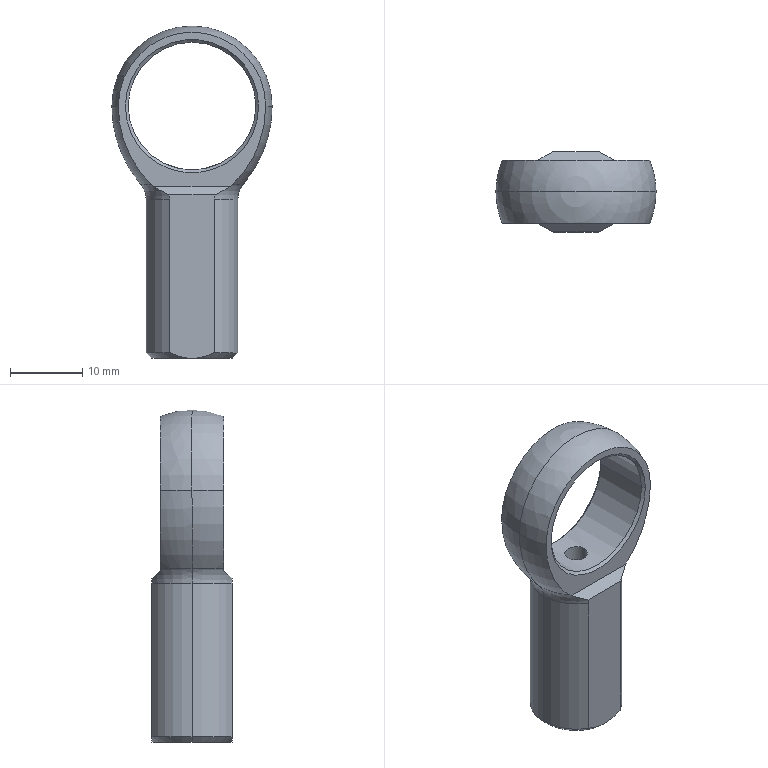Part | NX | features LUMP1 2 | 1 solid | 42 faces | box 22.225 x 11.1 x 46.038 mm | volume 3030 mm3 | cylinder 12 | cone 12 | plane 8 | torus 8 | sphere 2 | commonest cylinder face diameters 12.7 x4 3.175 x2 6.678 x2 7.938 x2 17.704 x2
STEP:
#1=CARTESIAN_POINT('',(3.339,0.,19.05));
#2=VERTEX_POINT('',#1);
#3=CARTESIAN_POINT('',(-3.339,0.,19.05));
#4=VERTEX_POINT('',#3);
#5=CARTESIAN_POINT('',(0.,0.,19.05));
#6=DIRECTION('',(0.,0.,-1.));
#7=DIRECTION('',(1.,0.,0.));
#8=AXIS2_PLACEMENT_3D('',#5,#6,#7);
#9=CIRCLE('',#8,3.339);
#10=EDGE_CURVE('',#2,#4,#9,.T.);
#11=ORIENTED_EDGE('',*,*,#10,.F.);
#12=CARTESIAN_POINT('',(0.,0.,19.05));
#13=DIRECTION('',(0.,0.,-1.));
#14=DIRECTION('',(1.,0.,0.));
#15=AXIS2_PLACEMENT_3D('',#12,#13,#14);
#16=CIRCLE('',#15,3.339);
#17=EDGE_CURVE('',#4,#2,#16,.T.);
#18=ORIENTED_EDGE('',*,*,#17,.F.);
#19=EDGE_LOOP('',(#11,#18));
#20=FACE_BOUND('',#19,.T.);
#21=CARTESIAN_POINT('',(3.969,0.,19.05));
#22=VERTEX_POINT('',#21);
#23=CARTESIAN_POINT('',(-3.969,0.,19.05));
#24=VERTEX_POINT('',#23);
#25=CARTESIAN_POINT('',(0.,0.,19.05));
#26=DIRECTION('',(0.,0.,1.));
#27=DIRECTION('',(1.,0.,0.));
#28=AXIS2_PLACEMENT_3D('',#25,#26,#27);
#29=CIRCLE('',#28,3.969);
#30=EDGE_CURVE('',#22,#24,#29,.T.);
#31=ORIENTED_EDGE('',*,*,#30,.F.);
#32=CARTESIAN_POINT('',(0.,0.,19.05));
#33=DIRECTION('',(0.,0.,1.));
#34=DIRECTION('',(1.,0.,0.));
#35=AXIS2_PLACEMENT_3D('',#32,#33,#34);
#36=CIRCLE('',#35,3.969);
#37=EDGE_CURVE('',#24,#22,#36,.T.);
#38=ORIENTED_EDGE('',*,*,#37,.F.);
#39=EDGE_LOOP('',(#31,#38));
#40=FACE_BOUND('',#39,.T.);
#41=CARTESIAN_POINT('',(0.,0.,19.05));
#42=DIRECTION('',(0.,0.,1.));
#43=DIRECTION('',(-1.,0.,0.));
#44=AXIS2_PLACEMENT_3D('',#41,#42,#43);
#45=PLANE('',#44);
#46=ADVANCED_FACE('',(#20,#40),#45,.F.);
#47=CARTESIAN_POINT('',(3.339,0.,22.225));
#48=VERTEX_POINT('',#47);
#49=CARTESIAN_POINT('',(3.339,0.,20.637));
#50=DIRECTION('',(0.,0.,1.));
#51=VECTOR('',#50,1000.);
#52=LINE('',#49,#51);
#53=EDGE_CURVE('',#2,#48,#52,.T.);
#54=ORIENTED_EDGE('',*,*,#53,.F.);
#55=ORIENTED_EDGE('',*,*,#10,.T.);
#56=CARTESIAN_POINT('',(-3.339,0.,22.225));
#57=VERTEX_POINT('',#56);
#58=CARTESIAN_POINT('',(-3.339,0.,20.637));
#59=DIRECTION('',(0.,0.,-1.));
#60=VECTOR('',#59,1000.);
#61=LINE('',#58,#60);
#62=EDGE_CURVE('',#57,#4,#61,.T.);
#63=ORIENTED_EDGE('',*,*,#62,.F.);
#64=CARTESIAN_POINT('',(0.,0.,22.225));
#65=DIRECTION('',(0.,0.,-1.));
#66=DIRECTION('',(1.,0.,0.));
#67=AXIS2_PLACEMENT_3D('',#64,#65,#66);
#68=CIRCLE('',#67,3.339);
#69=EDGE_CURVE('',#48,#57,#68,.T.);
#70=ORIENTED_EDGE('',*,*,#69,.F.);
#71=EDGE_LOOP('',(#54,#55,#63,#70));
#72=FACE_BOUND('',#71,.T.);
#73=CARTESIAN_POINT('',(0.,0.,20.637));
#74=DIRECTION('',(0.,0.,-1.));
#75=DIRECTION('',(-1.,0.,0.));
#76=AXIS2_PLACEMENT_3D('',#73,#74,#75);
#77=CYLINDRICAL_SURFACE('',#76,3.339);
#78=ADVANCED_FACE('',(#72),#77,.F.);
#79=ORIENTED_EDGE('',*,*,#53,.T.);
#80=CARTESIAN_POINT('',(0.,0.,22.225));
#81=DIRECTION('',(0.,0.,-1.));
#82=DIRECTION('',(1.,0.,0.));
#83=AXIS2_PLACEMENT_3D('',#80,#81,#82);
#84=CIRCLE('',#83,3.339);
#85=EDGE_CURVE('',#57,#48,#84,.T.);
#86=ORIENTED_EDGE('',*,*,#85,.F.);
#87=ORIENTED_EDGE('',*,*,#62,.T.);
#88=ORIENTED_EDGE('',*,*,#17,.T.);
#89=EDGE_LOOP('',(#79,#86,#87,#88));
#90=FACE_BOUND('',#89,.T.);
#91=CARTESIAN_POINT('',(0.,0.,20.637));
#92=DIRECTION('',(0.,0.,-1.));
#93=DIRECTION('',(-1.,0.,0.));
#94=AXIS2_PLACEMENT_3D('',#91,#92,#93);
#95=CYLINDRICAL_SURFACE('',#94,3.339);
#96=ADVANCED_FACE('',(#90),#95,.F.);
#97=CARTESIAN_POINT('',(3.969,0.,0.1321));
#98=VERTEX_POINT('',#97);
#99=CARTESIAN_POINT('',(3.969,0.,9.525));
#100=DIRECTION('',(0.,0.,-1.));
#101=VECTOR('',#100,1000.);
#102=LINE('',#99,#101);
#103=EDGE_CURVE('',#22,#98,#102,.T.);
#104=ORIENTED_EDGE('',*,*,#103,.F.);
#105=ORIENTED_EDGE('',*,*,#30,.T.);
#106=CARTESIAN_POINT('',(-3.969,0.,0.1321));
#107=VERTEX_POINT('',#106);
#108=CARTESIAN_POINT('',(-3.969,0.,9.525));
#109=DIRECTION('',(0.,0.,1.));
#110=VECTOR('',#109,1000.);
#111=LINE('',#108,#110);
#112=EDGE_CURVE('',#107,#24,#111,.T.);
#113=ORIENTED_EDGE('',*,*,#112,.F.);
#114=CARTESIAN_POINT('',(0.,0.,0.1321));
#115=DIRECTION('',(0.,0.,-1.));
#116=DIRECTION('',(1.,0.,0.));
#117=AXIS2_PLACEMENT_3D('',#114,#115,#116);
#118=CIRCLE('',#117,3.969);
#119=EDGE_CURVE('',#107,#98,#118,.T.);
#120=ORIENTED_EDGE('',*,*,#119,.T.);
#121=EDGE_LOOP('',(#104,#105,#113,#120));
#122=FACE_BOUND('',#121,.T.);
#123=CARTESIAN_POINT('',(0.,0.,9.525));
#124=DIRECTION('',(0.,0.,1.));
#125=DIRECTION('',(-1.,0.,0.));
#126=AXIS2_PLACEMENT_3D('',#123,#124,#125);
#127=CYLINDRICAL_SURFACE('',#126,3.969);
#128=ADVANCED_FACE('',(#122),#127,.F.);
#129=ORIENTED_EDGE('',*,*,#103,.T.);
#130=CARTESIAN_POINT('',(0.,0.,0.1321));
#131=DIRECTION('',(0.,0.,-1.));
#132=DIRECTION('',(1.,0.,0.));
#133=AXIS2_PLACEMENT_3D('',#130,#131,#132);
#134=CIRCLE('',#133,3.969);
#135=EDGE_CURVE('',#98,#107,#134,.T.);
#136=ORIENTED_EDGE('',*,*,#135,.T.);
#137=ORIENTED_EDGE('',*,*,#112,.T.);
#138=ORIENTED_EDGE('',*,*,#37,.T.);
#139=EDGE_LOOP('',(#129,#136,#137,#138));
#140=FACE_BOUND('',#139,.T.);
#141=CARTESIAN_POINT('',(0.,0.,9.525));
#142=DIRECTION('',(0.,0.,1.));
#143=DIRECTION('',(-1.,0.,0.));
#144=AXIS2_PLACEMENT_3D('',#141,#142,#143);
#145=CYLINDRICAL_SURFACE('',#144,3.969);
#146=ADVANCED_FACE('',(#140),#145,.F.);
#147=CARTESIAN_POINT('',(1.587,0.,23.236));
#148=VERTEX_POINT('',#147);
#149=CARTESIAN_POINT('',(1.669,0.,23.189));
#150=DIRECTION('',(-0.866,0.,0.5));
#151=VECTOR('',#150,1000.);
#152=LINE('',#149,#151);
#153=EDGE_CURVE('',#48,#148,#152,.T.);
#154=ORIENTED_EDGE('',*,*,#153,.F.);
#155=ORIENTED_EDGE('',*,*,#69,.T.);
#156=CARTESIAN_POINT('',(-1.587,0.,23.236));
#157=VERTEX_POINT('',#156);
#158=CARTESIAN_POINT('',(-1.669,0.,23.189));
#159=DIRECTION('',(-0.866,0.,-0.5));
#160=VECTOR('',#159,1000.);
#161=LINE('',#158,#160);
#162=EDGE_CURVE('',#157,#57,#161,.T.);
#163=ORIENTED_EDGE('',*,*,#162,.F.);
#164=CARTESIAN_POINT('',(-1.587,0.,23.236));
#165=CARTESIAN_POINT('',(-1.587,-0.2032,23.236));
#166=CARTESIAN_POINT('',(-1.548,-0.4045,23.236));
#167=CARTESIAN_POINT('',(-1.395,-0.7848,23.236));
#168=CARTESIAN_POINT('',(-1.281,-0.9596,23.236));
#169=CARTESIAN_POINT('',(-0.9929,-1.256,23.236));
#170=CARTESIAN_POINT('',(-0.8211,-1.374,23.236));
#171=CARTESIAN_POINT('',(-0.4418,-1.539,23.236));
#172=CARTESIAN_POINT('',(-0.2379,-1.583,23.236));
#173=CARTESIAN_POINT('',(0.1754,-1.591,23.236));
#174=CARTESIAN_POINT('',(0.3809,-1.555,23.236));
#175=CARTESIAN_POINT('',(0.7664,-1.406,23.236));
#176=CARTESIAN_POINT('',(0.9427,-1.294,23.236));
#177=CARTESIAN_POINT('',(1.243,-1.009,23.236));
#178=CARTESIAN_POINT('',(1.363,-0.8391,23.236));
#179=CARTESIAN_POINT('',(1.533,-0.462,23.236));
#180=CARTESIAN_POINT('',(1.58,-0.2587,23.236));
#181=CARTESIAN_POINT('',(1.587,-0.03471,23.236));
#182=CARTESIAN_POINT('',(1.587,-0.01735,23.236));
#183=CARTESIAN_POINT('',(1.587,0.,23.236));
#184=B_SPLINE_CURVE_WITH_KNOTS('',3,(#164,#165,#166,#167,#168,#169,#170,#171,#172,#173,#174,#175,#176,#177,#178,#179,#180,#181,#182,#183),.UNSPECIFIED.,.F.,.F.,(4,2,2,2,2,2,2,2,2,4),(0.,0.1219,0.2458,0.3698,0.4937,0.6177,0.7417,0.8656,0.9896,1.),.UNSPECIFIED.);
#185=EDGE_CURVE('',#157,#148,#184,.T.);
#186=ORIENTED_EDGE('',*,*,#185,.T.);
#187=EDGE_LOOP('',(#154,#155,#163,#186));
#188=FACE_BOUND('',#187,.T.);
#189=CARTESIAN_POINT('',(0.,0.,23.189));
#190=DIRECTION('',(0.,0.,-1.));
#191=DIRECTION('',(-1.,0.,0.));
#192=AXIS2_PLACEMENT_3D('',#189,#190,#191);
#193=CONICAL_SURFACE('',#192,1.669,1.047);
#194=ADVANCED_FACE('',(#188),#193,.F.);
#195=ORIENTED_EDGE('',*,*,#153,.T.);
#196=CARTESIAN_POINT('',(-1.123,1.123,23.236));
#197=VERTEX_POINT('',#196);
#198=CARTESIAN_POINT('',(1.587,0.,23.236));
#199=CARTESIAN_POINT('',(1.587,0.1891,23.236));
#200=CARTESIAN_POINT('',(1.554,0.3768,23.236));
#201=CARTESIAN_POINT('',(1.415,0.7479,23.236));
#202=CARTESIAN_POINT('',(1.306,0.9257,23.236));
#203=CARTESIAN_POINT('',(1.026,1.229,23.236));
#204=CARTESIAN_POINT('',(0.8569,1.352,23.236));
#205=CARTESIAN_POINT('',(0.4821,1.527,23.236));
#206=CARTESIAN_POINT('',(0.2794,1.576,23.236));
#207=CARTESIAN_POINT('',(-0.1336,1.595,23.236));
#208=CARTESIAN_POINT('',(-0.34,1.564,23.236));
#209=CARTESIAN_POINT('',(-0.6448,1.455,23.236));
#210=CARTESIAN_POINT('',(-0.7503,1.404,23.236));
#211=CARTESIAN_POINT('',(-0.9481,1.279,23.236));
#212=CARTESIAN_POINT('',(-1.04,1.205,23.236));
#213=CARTESIAN_POINT('',(-1.123,1.123,23.236));
#214=B_SPLINE_CURVE_WITH_KNOTS('',3,(#198,#199,#200,#201,#202,#203,#204,#205,#206,#207,#208,#209,#210,#211,#212,#213),.UNSPECIFIED.,.F.,.F.,(4,2,2,2,2,2,2,4),(0.,0.1514,0.3168,0.4821,0.6474,0.8128,0.9064,1.),.UNSPECIFIED.);
#215=EDGE_CURVE('',#148,#197,#214,.T.);
#216=ORIENTED_EDGE('',*,*,#215,.T.);
#217=CARTESIAN_POINT('',(-1.123,1.123,23.236));
#218=CARTESIAN_POINT('',(-1.269,0.9764,23.236));
#219=CARTESIAN_POINT('',(-1.385,0.803,23.236));
#220=CARTESIAN_POINT('',(-1.544,0.4216,23.236));
#221=CARTESIAN_POINT('',(-1.586,0.2171,23.236));
#222=CARTESIAN_POINT('',(-1.587,0.006944,23.236));
#223=CARTESIAN_POINT('',(-1.587,0.003472,23.236));
#224=CARTESIAN_POINT('',(-1.587,0.,23.236));
#225=B_SPLINE_CURVE_WITH_KNOTS('',3,(#217,#218,#219,#220,#221,#222,#223,#224),.UNSPECIFIED.,.F.,.F.,(4,2,2,4),(0.,0.4958,0.9917,1.),.UNSPECIFIED.);
#226=EDGE_CURVE('',#197,#157,#225,.T.);
#227=ORIENTED_EDGE('',*,*,#226,.T.);
#228=ORIENTED_EDGE('',*,*,#162,.T.);
#229=ORIENTED_EDGE('',*,*,#85,.T.);
#230=EDGE_LOOP('',(#195,#216,#227,#228,#229));
#231=FACE_BOUND('',#230,.T.);
#232=CARTESIAN_POINT('',(0.,0.,23.189));
#233=DIRECTION('',(0.,0.,-1.));
#234=DIRECTION('',(-1.,0.,0.));
#235=AXIS2_PLACEMENT_3D('',#232,#233,#234);
#236=CONICAL_SURFACE('',#235,1.669,1.047);
#237=ADVANCED_FACE('',(#231),#236,.F.);
#238=CARTESIAN_POINT('',(-4.101,0.,0.));
#239=VERTEX_POINT('',#238);
#240=CARTESIAN_POINT('',(-3.72,0.,0.381));
#241=DIRECTION('',(0.7071,0.,0.7071));
#242=VECTOR('',#241,1000.);
#243=LINE('',#240,#242);
#244=EDGE_CURVE('',#239,#107,#243,.T.);
#245=ORIENTED_EDGE('',*,*,#244,.F.);
#246=CARTESIAN_POINT('',(4.101,0.,0.));
#247=VERTEX_POINT('',#246);
#248=CARTESIAN_POINT('',(0.,0.,0.));
#249=DIRECTION('',(0.,0.,1.));
#250=DIRECTION('',(-1.,0.,0.));
#251=AXIS2_PLACEMENT_3D('',#248,#249,#250);
#252=CIRCLE('',#251,4.101);
#253=EDGE_CURVE('',#247,#239,#252,.T.);
#254=ORIENTED_EDGE('',*,*,#253,.F.);
#255=CARTESIAN_POINT('',(3.72,0.,0.381));
#256=DIRECTION('',(0.7071,0.,-0.7071));
#257=VECTOR('',#256,1000.);
#258=LINE('',#255,#257);
#259=EDGE_CURVE('',#98,#247,#258,.T.);
#260=ORIENTED_EDGE('',*,*,#259,.F.);
#261=ORIENTED_EDGE('',*,*,#119,.F.);
#262=EDGE_LOOP('',(#245,#254,#260,#261));
#263=FACE_BOUND('',#262,.T.);
#264=CARTESIAN_POINT('',(0.,0.,0.381));
#265=DIRECTION('',(0.,0.,-1.));
#266=DIRECTION('',(1.,0.,0.));
#267=AXIS2_PLACEMENT_3D('',#264,#265,#266);
#268=CONICAL_SURFACE('',#267,3.72,0.7854);
#269=ADVANCED_FACE('',(#263),#268,.F.);
#270=ORIENTED_EDGE('',*,*,#244,.T.);
#271=ORIENTED_EDGE('',*,*,#135,.F.);
#272=ORIENTED_EDGE('',*,*,#259,.T.);
#273=CARTESIAN_POINT('',(0.,0.,0.));
#274=DIRECTION('',(0.,0.,1.));
#275=DIRECTION('',(-1.,0.,0.));
#276=AXIS2_PLACEMENT_3D('',#273,#274,#275);
#277=CIRCLE('',#276,4.101);
#278=EDGE_CURVE('',#239,#247,#277,.T.);
#279=ORIENTED_EDGE('',*,*,#278,.F.);
#280=EDGE_LOOP('',(#270,#271,#272,#279));
#281=FACE_BOUND('',#280,.T.);
#282=CARTESIAN_POINT('',(0.,0.,0.381));
#283=DIRECTION('',(0.,0.,-1.));
#284=DIRECTION('',(1.,0.,0.));
#285=AXIS2_PLACEMENT_3D('',#282,#283,#284);
#286=CONICAL_SURFACE('',#285,3.72,0.7854);
#287=ADVANCED_FACE('',(#281),#286,.F.);
#288=CARTESIAN_POINT('',(1.587,0.,26.217));
#289=VERTEX_POINT('',#288);
#290=CARTESIAN_POINT('',(1.587,0.,17.462));
#291=DIRECTION('',(0.,0.,-1.));
#292=VECTOR('',#291,1000.);
#293=LINE('',#290,#292);
#294=EDGE_CURVE('',#289,#148,#293,.T.);
#295=ORIENTED_EDGE('',*,*,#294,.T.);
#296=ORIENTED_EDGE('',*,*,#185,.F.);
#297=CARTESIAN_POINT('',(-1.587,0.,26.217));
#298=VERTEX_POINT('',#297);
#299=CARTESIAN_POINT('',(-1.587,0.,17.462));
#300=DIRECTION('',(0.,0.,1.));
#301=VECTOR('',#300,1000.);
#302=LINE('',#299,#301);
#303=EDGE_CURVE('',#157,#298,#302,.T.);
#304=ORIENTED_EDGE('',*,*,#303,.T.);
#305=CARTESIAN_POINT('',(1.587,0.,26.217));
#306=CARTESIAN_POINT('',(1.587,-0.4204,26.217));
#307=CARTESIAN_POINT('',(1.243,-1.241,26.144));
#308=CARTESIAN_POINT('',(0.001873,-1.76,26.038));
#309=CARTESIAN_POINT('',(-1.243,-1.242,26.144));
#310=CARTESIAN_POINT('',(-1.587,-0.4204,26.217));
#311=CARTESIAN_POINT('',(-1.587,0.,26.217));
#312=B_SPLINE_CURVE_WITH_KNOTS('',3,(#305,#306,#307,#308,#309,#310,#311),.UNSPECIFIED.,.F.,.F.,(4,1,1,1,4),(0.,0.001243,0.002486,0.003729,0.004972),.UNSPECIFIED.);
#313=EDGE_CURVE('',#289,#298,#312,.T.);
#314=ORIENTED_EDGE('',*,*,#313,.F.);
#315=EDGE_LOOP('',(#295,#296,#304,#314));
#316=FACE_BOUND('',#315,.T.);
#317=CARTESIAN_POINT('',(0.,0.,17.462));
#318=DIRECTION('',(0.,0.,1.));
#319=DIRECTION('',(-1.,0.,0.));
#320=AXIS2_PLACEMENT_3D('',#317,#318,#319);
#321=CYLINDRICAL_SURFACE('',#320,1.587);
#322=ADVANCED_FACE('',(#316),#321,.F.);
#323=ORIENTED_EDGE('',*,*,#294,.F.);
#324=CARTESIAN_POINT('',(-1.587,0.,26.217));
#325=CARTESIAN_POINT('',(-1.587,0.4204,26.217));
#326=CARTESIAN_POINT('',(-1.243,1.241,26.144));
#327=CARTESIAN_POINT('',(-0.001873,1.76,26.038));
#328=CARTESIAN_POINT('',(1.243,1.242,26.144));
#329=CARTESIAN_POINT('',(1.587,0.4204,26.217));
#330=CARTESIAN_POINT('',(1.587,0.,26.217));
#331=B_SPLINE_CURVE_WITH_KNOTS('',3,(#324,#325,#326,#327,#328,#329,#330),.UNSPECIFIED.,.F.,.F.,(4,1,1,1,4),(0.,0.001243,0.002486,0.003729,0.004972),.UNSPECIFIED.);
#332=EDGE_CURVE('',#298,#289,#331,.T.);
#333=ORIENTED_EDGE('',*,*,#332,.F.);
#334=ORIENTED_EDGE('',*,*,#303,.F.);
#335=ORIENTED_EDGE('',*,*,#226,.F.);
#336=ORIENTED_EDGE('',*,*,#215,.F.);
#337=EDGE_LOOP('',(#323,#333,#334,#335,#336));
#338=FACE_BOUND('',#337,.T.);
#339=CARTESIAN_POINT('',(0.,0.,17.462));
#340=DIRECTION('',(0.,0.,1.));
#341=DIRECTION('',(-1.,0.,0.));
#342=AXIS2_PLACEMENT_3D('',#339,#340,#341);
#343=CYLINDRICAL_SURFACE('',#342,1.587);
#344=ADVANCED_FACE('',(#338),#343,.F.);
#345=CARTESIAN_POINT('',(6.35,0.,0.762));
#346=VERTEX_POINT('',#345);
#347=CARTESIAN_POINT('',(6.35,0.,22.028));
#348=VERTEX_POINT('',#347);
#349=CARTESIAN_POINT('',(6.35,0.,11.014));
#350=DIRECTION('',(0.,0.,1.));
#351=VECTOR('',#350,1000.);
#352=LINE('',#349,#351);
#353=EDGE_CURVE('',#346,#348,#352,.T.);
#354=ORIENTED_EDGE('',*,*,#353,.T.);
#355=CARTESIAN_POINT('',(3.086,-5.55,22.028));
#356=VERTEX_POINT('',#355);
#357=CARTESIAN_POINT('',(0.,0.,22.028));
#358=DIRECTION('',(0.,0.,-1.));
#359=DIRECTION('',(1.,0.,0.));
#360=AXIS2_PLACEMENT_3D('',#357,#358,#359);
#361=CIRCLE('',#360,6.35);
#362=EDGE_CURVE('',#348,#356,#361,.T.);
#363=ORIENTED_EDGE('',*,*,#362,.T.);
#364=CARTESIAN_POINT('',(3.086,-5.55,0.762));
#365=VERTEX_POINT('',#364);
#366=CARTESIAN_POINT('',(3.086,-5.55,11.014));
#367=DIRECTION('',(0.,0.,-1.));
#368=VECTOR('',#367,1000.);
#369=LINE('',#366,#368);
#370=EDGE_CURVE('',#356,#365,#369,.T.);
#371=ORIENTED_EDGE('',*,*,#370,.T.);
#372=CARTESIAN_POINT('',(0.,0.,0.762));
#373=DIRECTION('',(0.,0.,1.));
#374=DIRECTION('',(1.,0.,0.));
#375=AXIS2_PLACEMENT_3D('',#372,#373,#374);
#376=CIRCLE('',#375,6.35);
#377=EDGE_CURVE('',#365,#346,#376,.T.);
#378=ORIENTED_EDGE('',*,*,#377,.T.);
#379=EDGE_LOOP('',(#354,#363,#371,#378));
#380=FACE_BOUND('',#379,.T.);
#381=CARTESIAN_POINT('',(0.,0.,11.014));
#382=DIRECTION('',(0.,0.,1.));
#383=DIRECTION('',(-1.,0.,0.));
#384=AXIS2_PLACEMENT_3D('',#381,#382,#383);
#385=CYLINDRICAL_SURFACE('',#384,6.35);
#386=ADVANCED_FACE('',(#380),#385,.T.);
#387=CARTESIAN_POINT('',(5.588,0.,0.));
#388=VERTEX_POINT('',#387);
#389=CARTESIAN_POINT('',(5.969,0.,0.381));
#390=DIRECTION('',(0.7071,0.,0.7071));
#391=VECTOR('',#390,1000.);
#392=LINE('',#389,#391);
#393=EDGE_CURVE('',#388,#346,#392,.T.);
#394=ORIENTED_EDGE('',*,*,#393,.T.);
#395=ORIENTED_EDGE('',*,*,#377,.F.);
#396=CARTESIAN_POINT('',(0.6514,-5.55,0.));
#397=VERTEX_POINT('',#396);
#398=CARTESIAN_POINT('',(0.6514,-5.55,0.));
#399=CARTESIAN_POINT('',(1.791,-5.55,0.1328));
#400=CARTESIAN_POINT('',(3.086,-5.55,0.762));
#401=(BOUNDED_CURVE()B_SPLINE_CURVE(2,(#398,#399,#400),.UNSPECIFIED.,.F.,.F.)B_SPLINE_CURVE_WITH_KNOTS((3,3),(0.,1.),.PIECEWISE_BEZIER_KNOTS.)CURVE()GEOMETRIC_REPRESENTATION_ITEM()RATIONAL_B_SPLINE_CURVE((1.,1.021,1.))REPRESENTATION_ITEM(''));
#402=EDGE_CURVE('',#397,#365,#401,.T.);
#403=ORIENTED_EDGE('',*,*,#402,.F.);
#404=CARTESIAN_POINT('',(0.,0.,0.));
#405=DIRECTION('',(0.,0.,-1.));
#406=DIRECTION('',(1.,0.,0.));
#407=AXIS2_PLACEMENT_3D('',#404,#405,#406);
#408=CIRCLE('',#407,5.588);
#409=EDGE_CURVE('',#388,#397,#408,.T.);
#410=ORIENTED_EDGE('',*,*,#409,.F.);
#411=EDGE_LOOP('',(#394,#395,#403,#410));
#412=FACE_BOUND('',#411,.T.);
#413=CARTESIAN_POINT('',(0.,0.,0.381));
#414=DIRECTION('',(0.,0.,1.));
#415=DIRECTION('',(-1.,0.,0.));
#416=AXIS2_PLACEMENT_3D('',#413,#414,#415);
#417=CONICAL_SURFACE('',#416,5.969,0.7854);
#418=ADVANCED_FACE('',(#412),#417,.T.);
#419=CARTESIAN_POINT('',(-6.35,0.,0.762));
#420=VERTEX_POINT('',#419);
#421=CARTESIAN_POINT('',(-5.588,0.,0.));
#422=VERTEX_POINT('',#421);
#423=CARTESIAN_POINT('',(-5.969,0.,0.381));
#424=DIRECTION('',(0.7071,0.,-0.7071));
#425=VECTOR('',#424,1000.);
#426=LINE('',#423,#425);
#427=EDGE_CURVE('',#420,#422,#426,.T.);
#428=ORIENTED_EDGE('',*,*,#427,.T.);
#429=CARTESIAN_POINT('',(-0.6514,-5.55,0.));
#430=VERTEX_POINT('',#429);
#431=CARTESIAN_POINT('',(0.,0.,0.));
#432=DIRECTION('',(0.,0.,-1.));
#433=DIRECTION('',(1.,0.,0.));
#434=AXIS2_PLACEMENT_3D('',#431,#432,#433);
#435=CIRCLE('',#434,5.588);
#436=EDGE_CURVE('',#430,#422,#435,.T.);
#437=ORIENTED_EDGE('',*,*,#436,.F.);
#438=CARTESIAN_POINT('',(-3.086,-5.55,0.762));
#439=VERTEX_POINT('',#438);
#440=CARTESIAN_POINT('',(-3.086,-5.55,0.762));
#441=CARTESIAN_POINT('',(-1.791,-5.55,0.1328));
#442=CARTESIAN_POINT('',(-0.6514,-5.55,0.));
#443=(BOUNDED_CURVE()B_SPLINE_CURVE(2,(#440,#441,#442),.UNSPECIFIED.,.F.,.F.)B_SPLINE_CURVE_WITH_KNOTS((3,3),(0.,1.),.PIECEWISE_BEZIER_KNOTS.)CURVE()GEOMETRIC_REPRESENTATION_ITEM()RATIONAL_B_SPLINE_CURVE((1.,1.021,1.))REPRESENTATION_ITEM(''));
#444=EDGE_CURVE('',#439,#430,#443,.T.);
#445=ORIENTED_EDGE('',*,*,#444,.F.);
#446=CARTESIAN_POINT('',(0.,0.,0.762));
#447=DIRECTION('',(0.,0.,1.));
#448=DIRECTION('',(1.,0.,0.));
#449=AXIS2_PLACEMENT_3D('',#446,#447,#448);
#450=CIRCLE('',#449,6.35);
#451=EDGE_CURVE('',#420,#439,#450,.T.);
#452=ORIENTED_EDGE('',*,*,#451,.F.);
#453=EDGE_LOOP('',(#428,#437,#445,#452));
#454=FACE_BOUND('',#453,.T.);
#455=CARTESIAN_POINT('',(0.,0.,0.381));
#456=DIRECTION('',(0.,0.,1.));
#457=DIRECTION('',(-1.,0.,0.));
#458=AXIS2_PLACEMENT_3D('',#455,#456,#457);
#459=CONICAL_SURFACE('',#458,5.969,0.7854);
#460=ADVANCED_FACE('',(#454),#459,.T.);
#461=ORIENTED_EDGE('',*,*,#278,.T.);
#462=ORIENTED_EDGE('',*,*,#253,.T.);
#463=EDGE_LOOP('',(#461,#462));
#464=FACE_BOUND('',#463,.T.);
#465=ORIENTED_EDGE('',*,*,#436,.T.);
#466=CARTESIAN_POINT('',(-0.6514,5.55,0.));
#467=VERTEX_POINT('',#466);
#468=CARTESIAN_POINT('',(0.,0.,0.));
#469=DIRECTION('',(0.,0.,-1.));
#470=DIRECTION('',(1.,0.,0.));
#471=AXIS2_PLACEMENT_3D('',#468,#469,#470);
#472=CIRCLE('',#471,5.588);
#473=EDGE_CURVE('',#422,#467,#472,.T.);
#474=ORIENTED_EDGE('',*,*,#473,.T.);
#475=CARTESIAN_POINT('',(0.6514,5.55,0.));
#476=VERTEX_POINT('',#475);
#477=CARTESIAN_POINT('',(0.,5.55,0.));
#478=DIRECTION('',(1.,0.,0.));
#479=VECTOR('',#478,1000.);
#480=LINE('',#477,#479);
#481=EDGE_CURVE('',#467,#476,#480,.T.);
#482=ORIENTED_EDGE('',*,*,#481,.T.);
#483=CARTESIAN_POINT('',(0.,0.,0.));
#484=DIRECTION('',(0.,0.,-1.));
#485=DIRECTION('',(1.,0.,0.));
#486=AXIS2_PLACEMENT_3D('',#483,#484,#485);
#487=CIRCLE('',#486,5.588);
#488=EDGE_CURVE('',#476,#388,#487,.T.);
#489=ORIENTED_EDGE('',*,*,#488,.T.);
#490=ORIENTED_EDGE('',*,*,#409,.T.);
#491=CARTESIAN_POINT('',(0.,-5.55,0.));
#492=DIRECTION('',(-1.,0.,0.));
#493=VECTOR('',#492,1000.);
#494=LINE('',#491,#493);
#495=EDGE_CURVE('',#397,#430,#494,.T.);
#496=ORIENTED_EDGE('',*,*,#495,.T.);
#497=EDGE_LOOP('',(#465,#474,#482,#489,#490,#496));
#498=FACE_BOUND('',#497,.T.);
#499=CARTESIAN_POINT('',(0.,0.,0.));
#500=DIRECTION('',(0.,0.,-1.));
#501=DIRECTION('',(-1.,0.,0.));
#502=AXIS2_PLACEMENT_3D('',#499,#500,#501);
#503=PLANE('',#502);
#504=ADVANCED_FACE('',(#464,#498),#503,.T.);
#505=ORIENTED_EDGE('',*,*,#393,.F.);
#506=ORIENTED_EDGE('',*,*,#488,.F.);
#507=CARTESIAN_POINT('',(3.086,5.55,0.762));
#508=VERTEX_POINT('',#507);
#509=CARTESIAN_POINT('',(3.086,5.55,0.762));
#510=CARTESIAN_POINT('',(1.791,5.55,0.1328));
#511=CARTESIAN_POINT('',(0.6514,5.55,0.));
#512=(BOUNDED_CURVE()B_SPLINE_CURVE(2,(#509,#510,#511),.UNSPECIFIED.,.F.,.F.)B_SPLINE_CURVE_WITH_KNOTS((3,3),(0.,1.),.PIECEWISE_BEZIER_KNOTS.)CURVE()GEOMETRIC_REPRESENTATION_ITEM()RATIONAL_B_SPLINE_CURVE((1.,1.021,1.))REPRESENTATION_ITEM(''));
#513=EDGE_CURVE('',#508,#476,#512,.T.);
#514=ORIENTED_EDGE('',*,*,#513,.F.);
#515=CARTESIAN_POINT('',(0.,0.,0.762));
#516=DIRECTION('',(0.,0.,1.));
#517=DIRECTION('',(1.,0.,0.));
#518=AXIS2_PLACEMENT_3D('',#515,#516,#517);
#519=CIRCLE('',#518,6.35);
#520=EDGE_CURVE('',#346,#508,#519,.T.);
#521=ORIENTED_EDGE('',*,*,#520,.F.);
#522=EDGE_LOOP('',(#505,#506,#514,#521));
#523=FACE_BOUND('',#522,.T.);
#524=CARTESIAN_POINT('',(0.,0.,0.381));
#525=DIRECTION('',(0.,0.,1.));
#526=DIRECTION('',(-1.,0.,0.));
#527=AXIS2_PLACEMENT_3D('',#524,#525,#526);
#528=CONICAL_SURFACE('',#527,5.969,0.7854);
#529=ADVANCED_FACE('',(#523),#528,.T.);
#530=ORIENTED_EDGE('',*,*,#427,.F.);
#531=CARTESIAN_POINT('',(-3.086,5.55,0.762));
#532=VERTEX_POINT('',#531);
#533=CARTESIAN_POINT('',(0.,0.,0.762));
#534=DIRECTION('',(0.,0.,1.));
#535=DIRECTION('',(1.,0.,0.));
#536=AXIS2_PLACEMENT_3D('',#533,#534,#535);
#537=CIRCLE('',#536,6.35);
#538=EDGE_CURVE('',#532,#420,#537,.T.);
#539=ORIENTED_EDGE('',*,*,#538,.F.);
#540=CARTESIAN_POINT('',(-0.6514,5.55,0.));
#541=CARTESIAN_POINT('',(-1.791,5.55,0.1328));
#542=CARTESIAN_POINT('',(-3.086,5.55,0.762));
#543=(BOUNDED_CURVE()B_SPLINE_CURVE(2,(#540,#541,#542),.UNSPECIFIED.,.F.,.F.)B_SPLINE_CURVE_WITH_KNOTS((3,3),(0.,1.),.PIECEWISE_BEZIER_KNOTS.)CURVE()GEOMETRIC_REPRESENTATION_ITEM()RATIONAL_B_SPLINE_CURVE((1.,1.021,1.))REPRESENTATION_ITEM(''));
#544=EDGE_CURVE('',#467,#532,#543,.T.);
#545=ORIENTED_EDGE('',*,*,#544,.F.);
#546=ORIENTED_EDGE('',*,*,#473,.F.);
#547=EDGE_LOOP('',(#530,#539,#545,#546));
#548=FACE_BOUND('',#547,.T.);
#549=CARTESIAN_POINT('',(0.,0.,0.381));
#550=DIRECTION('',(0.,0.,1.));
#551=DIRECTION('',(-1.,0.,0.));
#552=AXIS2_PLACEMENT_3D('',#549,#550,#551);
#553=CONICAL_SURFACE('',#552,5.969,0.7854);
#554=ADVANCED_FACE('',(#548),#553,.T.);
#555=ORIENTED_EDGE('',*,*,#353,.F.);
#556=ORIENTED_EDGE('',*,*,#520,.T.);
#557=CARTESIAN_POINT('',(3.086,5.55,22.028));
#558=VERTEX_POINT('',#557);
#559=CARTESIAN_POINT('',(3.086,5.55,11.014));
#560=DIRECTION('',(0.,0.,1.));
#561=VECTOR('',#560,1000.);
#562=LINE('',#559,#561);
#563=EDGE_CURVE('',#508,#558,#562,.T.);
#564=ORIENTED_EDGE('',*,*,#563,.T.);
#565=CARTESIAN_POINT('',(0.,0.,22.028));
#566=DIRECTION('',(0.,0.,-1.));
#567=DIRECTION('',(1.,0.,0.));
#568=AXIS2_PLACEMENT_3D('',#565,#566,#567);
#569=CIRCLE('',#568,6.35);
#570=EDGE_CURVE('',#558,#348,#569,.T.);
#571=ORIENTED_EDGE('',*,*,#570,.T.);
#572=EDGE_LOOP('',(#555,#556,#564,#571));
#573=FACE_BOUND('',#572,.T.);
#574=CARTESIAN_POINT('',(0.,0.,11.014));
#575=DIRECTION('',(0.,0.,1.));
#576=DIRECTION('',(-1.,0.,0.));
#577=AXIS2_PLACEMENT_3D('',#574,#575,#576);
#578=CYLINDRICAL_SURFACE('',#577,6.35);
#579=ADVANCED_FACE('',(#573),#578,.T.);
#580=CARTESIAN_POINT('',(8.852,-3.988,34.925));
#581=VERTEX_POINT('',#580);
#582=CARTESIAN_POINT('',(8.852,3.988,34.925));
#583=VERTEX_POINT('',#582);
#584=CARTESIAN_POINT('',(8.852,0.,34.925));
#585=DIRECTION('',(0.,1.,0.));
#586=VECTOR('',#585,1000.);
#587=LINE('',#584,#586);
#588=EDGE_CURVE('',#581,#583,#587,.T.);
#589=ORIENTED_EDGE('',*,*,#588,.T.);
#590=CARTESIAN_POINT('',(-8.852,3.988,34.925));
#591=VERTEX_POINT('',#590);
#592=CARTESIAN_POINT('',(0.,3.988,34.925));
#593=DIRECTION('',(0.,1.,0.));
#594=DIRECTION('',(1.,0.,0.));
#595=AXIS2_PLACEMENT_3D('',#592,#593,#594);
#596=CIRCLE('',#595,8.852);
#597=EDGE_CURVE('',#583,#591,#596,.T.);
#598=ORIENTED_EDGE('',*,*,#597,.T.);
#599=CARTESIAN_POINT('',(-8.852,-3.988,34.925));
#600=VERTEX_POINT('',#599);
#601=CARTESIAN_POINT('',(-8.852,0.,34.925));
#602=DIRECTION('',(0.,-1.,0.));
#603=VECTOR('',#602,1000.);
#604=LINE('',#601,#603);
#605=EDGE_CURVE('',#591,#600,#604,.T.);
#606=ORIENTED_EDGE('',*,*,#605,.T.);
#607=CARTESIAN_POINT('',(0.,-3.988,34.925));
#608=DIRECTION('',(0.,-1.,0.));
#609=DIRECTION('',(1.,0.,0.));
#610=AXIS2_PLACEMENT_3D('',#607,#608,#609);
#611=CIRCLE('',#610,8.852);
#612=EDGE_CURVE('',#600,#581,#611,.T.);
#613=ORIENTED_EDGE('',*,*,#612,.T.);
#614=EDGE_LOOP('',(#589,#598,#606,#613));
#615=FACE_BOUND('',#614,.T.);
#616=ORIENTED_EDGE('',*,*,#332,.T.);
#617=ORIENTED_EDGE('',*,*,#313,.T.);
#618=EDGE_LOOP('',(#616,#617));
#619=FACE_BOUND('',#618,.T.);
#620=CARTESIAN_POINT('',(0.,0.,34.925));
#621=DIRECTION('',(0.,-1.,0.));
#622=DIRECTION('',(-1.,0.,0.));
#623=AXIS2_PLACEMENT_3D('',#620,#621,#622);
#624=CYLINDRICAL_SURFACE('',#623,8.852);
#625=ADVANCED_FACE('',(#615,#619),#624,.F.);
#626=ORIENTED_EDGE('',*,*,#588,.F.);
#627=CARTESIAN_POINT('',(0.,-3.988,34.925));
#628=DIRECTION('',(0.,-1.,0.));
#629=DIRECTION('',(1.,0.,0.));
#630=AXIS2_PLACEMENT_3D('',#627,#628,#629);
#631=CIRCLE('',#630,8.852);
#632=EDGE_CURVE('',#581,#600,#631,.T.);
#633=ORIENTED_EDGE('',*,*,#632,.T.);
#634=ORIENTED_EDGE('',*,*,#605,.F.);
#635=CARTESIAN_POINT('',(0.,3.988,34.925));
#636=DIRECTION('',(0.,1.,0.));
#637=DIRECTION('',(1.,0.,0.));
#638=AXIS2_PLACEMENT_3D('',#635,#636,#637);
#639=CIRCLE('',#638,8.852);
#640=EDGE_CURVE('',#591,#583,#639,.T.);
#641=ORIENTED_EDGE('',*,*,#640,.T.);
#642=EDGE_LOOP('',(#626,#633,#634,#641));
#643=FACE_BOUND('',#642,.T.);
#644=CARTESIAN_POINT('',(0.,0.,34.925));
#645=DIRECTION('',(0.,-1.,0.));
#646=DIRECTION('',(-1.,0.,0.));
#647=AXIS2_PLACEMENT_3D('',#644,#645,#646);
#648=CYLINDRICAL_SURFACE('',#647,8.852);
#649=ADVANCED_FACE('',(#643),#648,.F.);
#650=CARTESIAN_POINT('',(7.112,0.,24.092));
#651=VERTEX_POINT('',#650);
#652=CARTESIAN_POINT('',(11.113,0.,34.925));
#653=VERTEX_POINT('',#652);
#654=CARTESIAN_POINT('',(-5.556,0.,34.925));
#655=DIRECTION('',(0.,-1.,0.));
#656=DIRECTION('',(1.,0.,0.));
#657=AXIS2_PLACEMENT_3D('',#654,#655,#656);
#658=CIRCLE('',#657,16.669);
#659=EDGE_CURVE('',#651,#653,#658,.T.);
#660=ORIENTED_EDGE('',*,*,#659,.T.);
#661=CARTESIAN_POINT('',(10.218,-4.369,34.925));
#662=VERTEX_POINT('',#661);
#663=CARTESIAN_POINT('',(0.,0.,34.925));
#664=DIRECTION('',(0.,0.,-1.));
#665=DIRECTION('',(1.,0.,0.));
#666=AXIS2_PLACEMENT_3D('',#663,#664,#665);
#667=CIRCLE('',#666,11.113);
#668=EDGE_CURVE('',#653,#662,#667,.T.);
#669=ORIENTED_EDGE('',*,*,#668,.T.);
#670=CARTESIAN_POINT('',(5.612,-4.369,24.092));
#671=VERTEX_POINT('',#670);
#672=CARTESIAN_POINT('',(10.218,-4.369,34.925));
#673=CARTESIAN_POINT('',(10.218,-4.369,32.888));
#674=CARTESIAN_POINT('',(9.41,-4.369,28.893));
#675=CARTESIAN_POINT('',(7.111,-4.369,25.475));
#676=CARTESIAN_POINT('',(5.612,-4.369,24.092));
#677=B_SPLINE_CURVE_WITH_KNOTS('',3,(#672,#673,#674,#675,#676),.UNSPECIFIED.,.F.,.F.,(4,1,4),(0.,0.006006,0.01201),.UNSPECIFIED.);
#678=EDGE_CURVE('',#662,#671,#677,.T.);
#679=ORIENTED_EDGE('',*,*,#678,.T.);
#680=CARTESIAN_POINT('',(0.,0.,24.092));
#681=DIRECTION('',(0.,0.,-1.));
#682=DIRECTION('',(1.,0.,0.));
#683=AXIS2_PLACEMENT_3D('',#680,#681,#682);
#684=CIRCLE('',#683,7.112);
#685=EDGE_CURVE('',#651,#671,#684,.T.);
#686=ORIENTED_EDGE('',*,*,#685,.F.);
#687=EDGE_LOOP('',(#660,#669,#679,#686));
#688=FACE_BOUND('',#687,.T.);
#689=CARTESIAN_POINT('',(0.,0.,34.925));
#690=DIRECTION('',(0.,0.,-1.));
#691=DIRECTION('',(-1.,0.,0.));
#692=AXIS2_PLACEMENT_3D('',#689,#690,#691);
#693=DEGENERATE_TOROIDAL_SURFACE('',#692,5.556,16.669,.F.);
#694=ADVANCED_FACE('',(#688),#693,.F.);
#695=CARTESIAN_POINT('',(9.525,0.,22.028));
#696=DIRECTION('',(0.,-1.,0.));
#697=DIRECTION('',(1.,0.,0.));
#698=AXIS2_PLACEMENT_3D('',#695,#696,#697);
#699=CIRCLE('',#698,3.175);
#700=EDGE_CURVE('',#651,#348,#699,.T.);
#701=ORIENTED_EDGE('',*,*,#700,.F.);
#702=ORIENTED_EDGE('',*,*,#685,.T.);
#703=CARTESIAN_POINT('',(5.328,-4.369,23.8));
#704=VERTEX_POINT('',#703);
#705=CARTESIAN_POINT('',(5.612,-4.369,24.092));
#706=CARTESIAN_POINT('',(5.512,-4.369,23.999));
#707=CARTESIAN_POINT('',(5.417,-4.369,23.902));
#708=CARTESIAN_POINT('',(5.328,-4.369,23.8));
#709=B_SPLINE_CURVE_WITH_KNOTS('',3,(#705,#706,#707,#708),.UNSPECIFIED.,.F.,.F.,(4,4),(0.,0.000407),.UNSPECIFIED.);
#710=EDGE_CURVE('',#671,#704,#709,.T.);
#711=ORIENTED_EDGE('',*,*,#710,.T.);
#712=CARTESIAN_POINT('',(3.198,-5.55,22.619));
#713=VERTEX_POINT('',#712);
#714=CARTESIAN_POINT('',(5.328,-4.369,23.8));
#715=CARTESIAN_POINT('',(4.636,-4.779,23.39));
#716=CARTESIAN_POINT('',(3.95,-5.194,22.974));
#717=CARTESIAN_POINT('',(3.198,-5.55,22.619));
#718=B_SPLINE_CURVE_WITH_KNOTS('',3,(#714,#715,#716,#717),.UNSPECIFIED.,.F.,.F.,(4,4),(0.,0.002707),.UNSPECIFIED.);
#719=EDGE_CURVE('',#704,#713,#718,.T.);
#720=ORIENTED_EDGE('',*,*,#719,.T.);
#721=CARTESIAN_POINT('',(3.198,-5.55,22.619));
#722=CARTESIAN_POINT('',(3.126,-5.55,22.428));
#723=CARTESIAN_POINT('',(3.086,-5.55,22.232));
#724=CARTESIAN_POINT('',(3.086,-5.55,22.028));
#725=B_SPLINE_CURVE_WITH_KNOTS('',3,(#721,#722,#723,#724),.UNSPECIFIED.,.F.,.F.,(4,4),(0.,0.0006012),.UNSPECIFIED.);
#726=EDGE_CURVE('',#713,#356,#725,.T.);
#727=ORIENTED_EDGE('',*,*,#726,.T.);
#728=ORIENTED_EDGE('',*,*,#362,.F.);
#729=EDGE_LOOP('',(#701,#702,#711,#720,#727,#728));
#730=FACE_BOUND('',#729,.T.);
#731=CARTESIAN_POINT('',(0.,0.,22.028));
#732=DIRECTION('',(0.,0.,-1.));
#733=DIRECTION('',(1.,0.,0.));
#734=AXIS2_PLACEMENT_3D('',#731,#732,#733);
#735=TOROIDAL_SURFACE('',#734,9.525,3.175);
#736=ADVANCED_FACE('',(#730),#735,.F.);
#737=CARTESIAN_POINT('',(9.233,-4.369,34.925));
#738=VERTEX_POINT('',#737);
#739=CARTESIAN_POINT('',(9.042,-4.178,34.925));
#740=DIRECTION('',(-0.7071,0.7071,0.));
#741=VECTOR('',#740,1000.);
#742=LINE('',#739,#741);
#743=EDGE_CURVE('',#738,#581,#742,.T.);
#744=ORIENTED_EDGE('',*,*,#743,.F.);
#745=CARTESIAN_POINT('',(-9.233,-4.369,34.925));
#746=VERTEX_POINT('',#745);
#747=CARTESIAN_POINT('',(0.,-4.369,34.925));
#748=DIRECTION('',(0.,1.,0.));
#749=DIRECTION('',(1.,0.,0.));
#750=AXIS2_PLACEMENT_3D('',#747,#748,#749);
#751=CIRCLE('',#750,9.233);
#752=EDGE_CURVE('',#746,#738,#751,.T.);
#753=ORIENTED_EDGE('',*,*,#752,.F.);
#754=CARTESIAN_POINT('',(-9.042,-4.178,34.925));
#755=DIRECTION('',(-0.7071,-0.7071,0.));
#756=VECTOR('',#755,1000.);
#757=LINE('',#754,#756);
#758=EDGE_CURVE('',#600,#746,#757,.T.);
#759=ORIENTED_EDGE('',*,*,#758,.F.);
#760=ORIENTED_EDGE('',*,*,#632,.F.);
#761=EDGE_LOOP('',(#744,#753,#759,#760));
#762=FACE_BOUND('',#761,.T.);
#763=CARTESIAN_POINT('',(0.,-4.178,34.925));
#764=DIRECTION('',(0.,-1.,0.));
#765=DIRECTION('',(-1.,0.,0.));
#766=AXIS2_PLACEMENT_3D('',#763,#764,#765);
#767=CONICAL_SURFACE('',#766,9.042,0.7854);
#768=ADVANCED_FACE('',(#762),#767,.F.);
#769=ORIENTED_EDGE('',*,*,#743,.T.);
#770=ORIENTED_EDGE('',*,*,#612,.F.);
#771=ORIENTED_EDGE('',*,*,#758,.T.);
#772=CARTESIAN_POINT('',(0.,-4.369,34.925));
#773=DIRECTION('',(0.,1.,0.));
#774=DIRECTION('',(1.,0.,0.));
#775=AXIS2_PLACEMENT_3D('',#772,#773,#774);
#776=CIRCLE('',#775,9.233);
#777=EDGE_CURVE('',#738,#746,#776,.T.);
#778=ORIENTED_EDGE('',*,*,#777,.F.);
#779=EDGE_LOOP('',(#769,#770,#771,#778));
#780=FACE_BOUND('',#779,.T.);
#781=CARTESIAN_POINT('',(0.,-4.178,34.925));
#782=DIRECTION('',(0.,-1.,0.));
#783=DIRECTION('',(-1.,0.,0.));
#784=AXIS2_PLACEMENT_3D('',#781,#782,#783);
#785=CONICAL_SURFACE('',#784,9.042,0.7854);
#786=ADVANCED_FACE('',(#780),#785,.F.);
#787=CARTESIAN_POINT('',(-3.198,-5.55,22.619));
#788=VERTEX_POINT('',#787);
#789=CARTESIAN_POINT('',(5.556,-5.55,22.619));
#790=DIRECTION('',(1.,0.,0.));
#791=VECTOR('',#790,1000.);
#792=LINE('',#789,#791);
#793=EDGE_CURVE('',#788,#713,#792,.T.);
#794=ORIENTED_EDGE('',*,*,#793,.T.);
#795=ORIENTED_EDGE('',*,*,#719,.F.);
#796=CARTESIAN_POINT('',(-5.328,-4.369,23.8));
#797=VERTEX_POINT('',#796);
#798=CARTESIAN_POINT('',(11.113,-4.369,23.8));
#799=DIRECTION('',(-1.,0.,0.));
#800=VECTOR('',#799,1000.);
#801=LINE('',#798,#800);
#802=EDGE_CURVE('',#704,#797,#801,.T.);
#803=ORIENTED_EDGE('',*,*,#802,.T.);
#804=CARTESIAN_POINT('',(-3.198,-5.55,22.619));
#805=CARTESIAN_POINT('',(-3.95,-5.194,22.974));
#806=CARTESIAN_POINT('',(-4.636,-4.779,23.39));
#807=CARTESIAN_POINT('',(-5.328,-4.369,23.8));
#808=B_SPLINE_CURVE_WITH_KNOTS('',3,(#804,#805,#806,#807),.UNSPECIFIED.,.F.,.F.,(4,4),(0.,0.002707),.UNSPECIFIED.);
#809=EDGE_CURVE('',#788,#797,#808,.T.);
#810=ORIENTED_EDGE('',*,*,#809,.F.);
#811=EDGE_LOOP('',(#794,#795,#803,#810));
#812=FACE_BOUND('',#811,.T.);
#813=CARTESIAN_POINT('',(11.113,-9.981,18.187));
#814=DIRECTION('',(0.,0.7071,-0.7071));
#815=DIRECTION('',(-1.,0.,0.));
#816=AXIS2_PLACEMENT_3D('',#813,#814,#815);
#817=PLANE('',#816);
#818=ADVANCED_FACE('',(#812),#817,.F.);
#819=ORIENTED_EDGE('',*,*,#444,.T.);
#820=ORIENTED_EDGE('',*,*,#495,.F.);
#821=ORIENTED_EDGE('',*,*,#402,.T.);
#822=ORIENTED_EDGE('',*,*,#370,.F.);
#823=ORIENTED_EDGE('',*,*,#726,.F.);
#824=ORIENTED_EDGE('',*,*,#793,.F.);
#825=CARTESIAN_POINT('',(-3.086,-5.55,22.028));
#826=VERTEX_POINT('',#825);
#827=CARTESIAN_POINT('',(-3.086,-5.55,22.028));
#828=CARTESIAN_POINT('',(-3.086,-5.55,22.232));
#829=CARTESIAN_POINT('',(-3.126,-5.55,22.428));
#830=CARTESIAN_POINT('',(-3.198,-5.55,22.619));
#831=B_SPLINE_CURVE_WITH_KNOTS('',3,(#827,#828,#829,#830),.UNSPECIFIED.,.F.,.F.,(4,4),(0.,0.0006012),.UNSPECIFIED.);
#832=EDGE_CURVE('',#826,#788,#831,.T.);
#833=ORIENTED_EDGE('',*,*,#832,.F.);
#834=CARTESIAN_POINT('',(-3.086,-5.55,11.014));
#835=DIRECTION('',(0.,0.,1.));
#836=VECTOR('',#835,1000.);
#837=LINE('',#834,#836);
#838=EDGE_CURVE('',#439,#826,#837,.T.);
#839=ORIENTED_EDGE('',*,*,#838,.F.);
#840=EDGE_LOOP('',(#819,#820,#821,#822,#823,#824,#833,#839));
#841=FACE_BOUND('',#840,.T.);
#842=CARTESIAN_POINT('',(0.,-5.55,12.76));
#843=DIRECTION('',(0.,-1.,0.));
#844=DIRECTION('',(-1.,0.,0.));
#845=AXIS2_PLACEMENT_3D('',#842,#843,#844);
#846=PLANE('',#845);
#847=ADVANCED_FACE('',(#841),#846,.T.);
#848=CARTESIAN_POINT('',(-6.35,0.,22.028));
#849=VERTEX_POINT('',#848);
#850=CARTESIAN_POINT('',(-6.35,0.,11.014));
#851=DIRECTION('',(0.,0.,-1.));
#852=VECTOR('',#851,1000.);
#853=LINE('',#850,#852);
#854=EDGE_CURVE('',#849,#420,#853,.T.);
#855=ORIENTED_EDGE('',*,*,#854,.T.);
#856=ORIENTED_EDGE('',*,*,#451,.T.);
#857=ORIENTED_EDGE('',*,*,#838,.T.);
#858=CARTESIAN_POINT('',(0.,0.,22.028));
#859=DIRECTION('',(0.,0.,-1.));
#860=DIRECTION('',(1.,0.,0.));
#861=AXIS2_PLACEMENT_3D('',#858,#859,#860);
#862=CIRCLE('',#861,6.35);
#863=EDGE_CURVE('',#826,#849,#862,.T.);
#864=ORIENTED_EDGE('',*,*,#863,.T.);
#865=EDGE_LOOP('',(#855,#856,#857,#864));
#866=FACE_BOUND('',#865,.T.);
#867=CARTESIAN_POINT('',(0.,0.,11.014));
#868=DIRECTION('',(0.,0.,1.));
#869=DIRECTION('',(-1.,0.,0.));
#870=AXIS2_PLACEMENT_3D('',#867,#868,#869);
#871=CYLINDRICAL_SURFACE('',#870,6.35);
#872=ADVANCED_FACE('',(#866),#871,.T.);
#873=ORIENTED_EDGE('',*,*,#854,.F.);
#874=CARTESIAN_POINT('',(-3.086,5.55,22.028));
#875=VERTEX_POINT('',#874);
#876=CARTESIAN_POINT('',(0.,0.,22.028));
#877=DIRECTION('',(0.,0.,-1.));
#878=DIRECTION('',(1.,0.,0.));
#879=AXIS2_PLACEMENT_3D('',#876,#877,#878);
#880=CIRCLE('',#879,6.35);
#881=EDGE_CURVE('',#849,#875,#880,.T.);
#882=ORIENTED_EDGE('',*,*,#881,.T.);
#883=CARTESIAN_POINT('',(-3.086,5.55,11.014));
#884=DIRECTION('',(0.,0.,-1.));
#885=VECTOR('',#884,1000.);
#886=LINE('',#883,#885);
#887=EDGE_CURVE('',#875,#532,#886,.T.);
#888=ORIENTED_EDGE('',*,*,#887,.T.);
#889=ORIENTED_EDGE('',*,*,#538,.T.);
#890=EDGE_LOOP('',(#873,#882,#888,#889));
#891=FACE_BOUND('',#890,.T.);
#892=CARTESIAN_POINT('',(0.,0.,11.014));
#893=DIRECTION('',(0.,0.,1.));
#894=DIRECTION('',(-1.,0.,0.));
#895=AXIS2_PLACEMENT_3D('',#892,#893,#894);
#896=CYLINDRICAL_SURFACE('',#895,6.35);
#897=ADVANCED_FACE('',(#891),#896,.T.);
#898=ORIENTED_EDGE('',*,*,#544,.T.);
#899=ORIENTED_EDGE('',*,*,#887,.F.);
#900=CARTESIAN_POINT('',(-3.198,5.55,22.619));
#901=VERTEX_POINT('',#900);
#902=CARTESIAN_POINT('',(-3.198,5.55,22.619));
#903=CARTESIAN_POINT('',(-3.126,5.55,22.428));
#904=CARTESIAN_POINT('',(-3.086,5.55,22.232));
#905=CARTESIAN_POINT('',(-3.086,5.55,22.028));
#906=B_SPLINE_CURVE_WITH_KNOTS('',3,(#902,#903,#904,#905),.UNSPECIFIED.,.F.,.F.,(4,4),(0.,0.0006012),.UNSPECIFIED.);
#907=EDGE_CURVE('',#901,#875,#906,.T.);
#908=ORIENTED_EDGE('',*,*,#907,.F.);
#909=CARTESIAN_POINT('',(3.198,5.55,22.619));
#910=VERTEX_POINT('',#909);
#911=CARTESIAN_POINT('',(-5.556,5.55,22.619));
#912=DIRECTION('',(-1.,0.,0.));
#913=VECTOR('',#912,1000.);
#914=LINE('',#911,#913);
#915=EDGE_CURVE('',#910,#901,#914,.T.);
#916=ORIENTED_EDGE('',*,*,#915,.F.);
#917=CARTESIAN_POINT('',(3.086,5.55,22.028));
#918=CARTESIAN_POINT('',(3.086,5.55,22.232));
#919=CARTESIAN_POINT('',(3.126,5.55,22.428));
#920=CARTESIAN_POINT('',(3.198,5.55,22.619));
#921=B_SPLINE_CURVE_WITH_KNOTS('',3,(#917,#918,#919,#920),.UNSPECIFIED.,.F.,.F.,(4,4),(0.,0.0006012),.UNSPECIFIED.);
#922=EDGE_CURVE('',#558,#910,#921,.T.);
#923=ORIENTED_EDGE('',*,*,#922,.F.);
#924=ORIENTED_EDGE('',*,*,#563,.F.);
#925=ORIENTED_EDGE('',*,*,#513,.T.);
#926=ORIENTED_EDGE('',*,*,#481,.F.);
#927=EDGE_LOOP('',(#898,#899,#908,#916,#923,#924,#925,#926));
#928=FACE_BOUND('',#927,.T.);
#929=CARTESIAN_POINT('',(0.,5.55,12.76));
#930=DIRECTION('',(0.,1.,0.));
#931=DIRECTION('',(-1.,0.,0.));
#932=AXIS2_PLACEMENT_3D('',#929,#930,#931);
#933=PLANE('',#932);
#934=ADVANCED_FACE('',(#928),#933,.T.);
#935=ORIENTED_EDGE('',*,*,#915,.T.);
#936=CARTESIAN_POINT('',(-5.328,4.369,23.8));
#937=VERTEX_POINT('',#936);
#938=CARTESIAN_POINT('',(-5.328,4.369,23.8));
#939=CARTESIAN_POINT('',(-4.636,4.779,23.39));
#940=CARTESIAN_POINT('',(-3.95,5.194,22.974));
#941=CARTESIAN_POINT('',(-3.198,5.55,22.619));
#942=B_SPLINE_CURVE_WITH_KNOTS('',3,(#938,#939,#940,#941),.UNSPECIFIED.,.F.,.F.,(4,4),(0.,0.002707),.UNSPECIFIED.);
#943=EDGE_CURVE('',#937,#901,#942,.T.);
#944=ORIENTED_EDGE('',*,*,#943,.F.);
#945=CARTESIAN_POINT('',(5.328,4.369,23.8));
#946=VERTEX_POINT('',#945);
#947=CARTESIAN_POINT('',(-11.113,4.369,23.8));
#948=DIRECTION('',(1.,0.,0.));
#949=VECTOR('',#948,1000.);
#950=LINE('',#947,#949);
#951=EDGE_CURVE('',#937,#946,#950,.T.);
#952=ORIENTED_EDGE('',*,*,#951,.T.);
#953=CARTESIAN_POINT('',(3.198,5.55,22.619));
#954=CARTESIAN_POINT('',(3.95,5.194,22.974));
#955=CARTESIAN_POINT('',(4.636,4.779,23.39));
#956=CARTESIAN_POINT('',(5.328,4.369,23.8));
#957=B_SPLINE_CURVE_WITH_KNOTS('',3,(#953,#954,#955,#956),.UNSPECIFIED.,.F.,.F.,(4,4),(0.,0.002707),.UNSPECIFIED.);
#958=EDGE_CURVE('',#910,#946,#957,.T.);
#959=ORIENTED_EDGE('',*,*,#958,.F.);
#960=EDGE_LOOP('',(#935,#944,#952,#959));
#961=FACE_BOUND('',#960,.T.);
#962=CARTESIAN_POINT('',(-11.113,9.981,18.187));
#963=DIRECTION('',(0.,-0.7071,-0.7071));
#964=DIRECTION('',(-1.,0.,0.));
#965=AXIS2_PLACEMENT_3D('',#962,#963,#964);
#966=PLANE('',#965);
#967=ADVANCED_FACE('',(#961),#966,.F.);
#968=ORIENTED_EDGE('',*,*,#700,.T.);
#969=ORIENTED_EDGE('',*,*,#570,.F.);
#970=ORIENTED_EDGE('',*,*,#922,.T.);
#971=ORIENTED_EDGE('',*,*,#958,.T.);
#972=CARTESIAN_POINT('',(5.612,4.369,24.092));
#973=VERTEX_POINT('',#972);
#974=CARTESIAN_POINT('',(5.328,4.369,23.8));
#975=CARTESIAN_POINT('',(5.417,4.369,23.902));
#976=CARTESIAN_POINT('',(5.512,4.369,23.999));
#977=CARTESIAN_POINT('',(5.612,4.369,24.092));
#978=B_SPLINE_CURVE_WITH_KNOTS('',3,(#974,#975,#976,#977),.UNSPECIFIED.,.F.,.F.,(4,4),(0.,0.000407),.UNSPECIFIED.);
#979=EDGE_CURVE('',#946,#973,#978,.T.);
#980=ORIENTED_EDGE('',*,*,#979,.T.);
#981=CARTESIAN_POINT('',(0.,0.,24.092));
#982=DIRECTION('',(0.,0.,-1.));
#983=DIRECTION('',(1.,0.,0.));
#984=AXIS2_PLACEMENT_3D('',#981,#982,#983);
#985=CIRCLE('',#984,7.112);
#986=EDGE_CURVE('',#973,#651,#985,.T.);
#987=ORIENTED_EDGE('',*,*,#986,.T.);
#988=EDGE_LOOP('',(#968,#969,#970,#971,#980,#987));
#989=FACE_BOUND('',#988,.T.);
#990=CARTESIAN_POINT('',(0.,0.,22.028));
#991=DIRECTION('',(0.,0.,-1.));
#992=DIRECTION('',(1.,0.,0.));
#993=AXIS2_PLACEMENT_3D('',#990,#991,#992);
#994=TOROIDAL_SURFACE('',#993,9.525,3.175);
#995=ADVANCED_FACE('',(#989),#994,.F.);
#996=CARTESIAN_POINT('',(9.233,4.369,34.925));
#997=VERTEX_POINT('',#996);
#998=CARTESIAN_POINT('',(9.042,4.178,34.925));
#999=DIRECTION('',(-0.7071,-0.7071,0.));
#1000=VECTOR('',#999,1000.);
#1001=LINE('',#998,#1000);
#1002=EDGE_CURVE('',#997,#583,#1001,.T.);
#1003=ORIENTED_EDGE('',*,*,#1002,.F.);
#1004=CARTESIAN_POINT('',(-9.233,4.369,34.925));
#1005=VERTEX_POINT('',#1004);
#1006=CARTESIAN_POINT('',(0.,4.369,34.925));
#1007=DIRECTION('',(0.,-1.,0.));
#1008=DIRECTION('',(1.,0.,0.));
#1009=AXIS2_PLACEMENT_3D('',#1006,#1007,#1008);
#1010=CIRCLE('',#1009,9.233);
#1011=EDGE_CURVE('',#1005,#997,#1010,.T.);
#1012=ORIENTED_EDGE('',*,*,#1011,.F.);
#1013=CARTESIAN_POINT('',(-9.042,4.178,34.925));
#1014=DIRECTION('',(-0.7071,0.7071,0.));
#1015=VECTOR('',#1014,1000.);
#1016=LINE('',#1013,#1015);
#1017=EDGE_CURVE('',#591,#1005,#1016,.T.);
#1018=ORIENTED_EDGE('',*,*,#1017,.F.);
#1019=ORIENTED_EDGE('',*,*,#597,.F.);
#1020=EDGE_LOOP('',(#1003,#1012,#1018,#1019));
#1021=FACE_BOUND('',#1020,.T.);
#1022=CARTESIAN_POINT('',(0.,4.178,34.925));
#1023=DIRECTION('',(0.,1.,0.));
#1024=DIRECTION('',(-1.,0.,0.));
#1025=AXIS2_PLACEMENT_3D('',#1022,#1023,#1024);
#1026=CONICAL_SURFACE('',#1025,9.042,0.7854);
#1027=ADVANCED_FACE('',(#1021),#1026,.F.);
#1028=ORIENTED_EDGE('',*,*,#1002,.T.);
#1029=ORIENTED_EDGE('',*,*,#640,.F.);
#1030=ORIENTED_EDGE('',*,*,#1017,.T.);
#1031=CARTESIAN_POINT('',(0.,4.369,34.925));
#1032=DIRECTION('',(0.,-1.,0.));
#1033=DIRECTION('',(1.,0.,0.));
#1034=AXIS2_PLACEMENT_3D('',#1031,#1032,#1033);
#1035=CIRCLE('',#1034,9.233);
#1036=EDGE_CURVE('',#997,#1005,#1035,.T.);
#1037=ORIENTED_EDGE('',*,*,#1036,.F.);
#1038=EDGE_LOOP('',(#1028,#1029,#1030,#1037));
#1039=FACE_BOUND('',#1038,.T.);
#1040=CARTESIAN_POINT('',(0.,4.178,34.925));
#1041=DIRECTION('',(0.,1.,0.));
#1042=DIRECTION('',(-1.,0.,0.));
#1043=AXIS2_PLACEMENT_3D('',#1040,#1041,#1042);
#1044=CONICAL_SURFACE('',#1043,9.042,0.7854);
#1045=ADVANCED_FACE('',(#1039),#1044,.F.);
#1046=ORIENTED_EDGE('',*,*,#659,.F.);
#1047=ORIENTED_EDGE('',*,*,#986,.F.);
#1048=CARTESIAN_POINT('',(10.218,4.369,34.925));
#1049=VERTEX_POINT('',#1048);
#1050=CARTESIAN_POINT('',(5.612,4.369,24.092));
#1051=CARTESIAN_POINT('',(8.602,4.369,26.85));
#1052=CARTESIAN_POINT('',(10.218,4.369,30.863));
#1053=CARTESIAN_POINT('',(10.218,4.369,34.925));
#1054=B_SPLINE_CURVE_WITH_KNOTS('',3,(#1050,#1051,#1052,#1053),.UNSPECIFIED.,.F.,.F.,(4,4),(0.,0.01205),.UNSPECIFIED.);
#1055=EDGE_CURVE('',#973,#1049,#1054,.T.);
#1056=ORIENTED_EDGE('',*,*,#1055,.T.);
#1057=CARTESIAN_POINT('',(0.,0.,34.925));
#1058=DIRECTION('',(0.,0.,-1.));
#1059=DIRECTION('',(1.,0.,0.));
#1060=AXIS2_PLACEMENT_3D('',#1057,#1058,#1059);
#1061=CIRCLE('',#1060,11.113);
#1062=EDGE_CURVE('',#1049,#653,#1061,.T.);
#1063=ORIENTED_EDGE('',*,*,#1062,.T.);
#1064=EDGE_LOOP('',(#1046,#1047,#1056,#1063));
#1065=FACE_BOUND('',#1064,.T.);
#1066=CARTESIAN_POINT('',(0.,0.,34.925));
#1067=DIRECTION('',(0.,0.,-1.));
#1068=DIRECTION('',(-1.,0.,0.));
#1069=AXIS2_PLACEMENT_3D('',#1066,#1067,#1068);
#1070=DEGENERATE_TOROIDAL_SURFACE('',#1069,5.556,16.669,.F.);
#1071=ADVANCED_FACE('',(#1065),#1070,.F.);
#1072=CARTESIAN_POINT('',(0.,0.,46.038));
#1073=VERTEX_POINT('',#1072);
#1074=CARTESIAN_POINT('',(-11.113,0.,34.925));
#1075=VERTEX_POINT('',#1074);
#1076=CARTESIAN_POINT('',(0.,0.,34.925));
#1077=DIRECTION('',(0.,-1.,0.));
#1078=DIRECTION('',(0.,0.,1.));
#1079=AXIS2_PLACEMENT_3D('',#1076,#1077,#1078);
#1080=CIRCLE('',#1079,11.113);
#1081=EDGE_CURVE('',#1073,#1075,#1080,.T.);
#1082=ORIENTED_EDGE('',*,*,#1081,.T.);
#1083=CARTESIAN_POINT('',(-10.218,-4.369,34.925));
#1084=VERTEX_POINT('',#1083);
#1085=CARTESIAN_POINT('',(0.,0.,34.925));
#1086=DIRECTION('',(0.,0.,-1.));
#1087=DIRECTION('',(1.,0.,0.));
#1088=AXIS2_PLACEMENT_3D('',#1085,#1086,#1087);
#1089=CIRCLE('',#1088,11.113);
#1090=EDGE_CURVE('',#1084,#1075,#1089,.T.);
#1091=ORIENTED_EDGE('',*,*,#1090,.F.);
#1092=CARTESIAN_POINT('',(0.,-4.369,34.925));
#1093=DIRECTION('',(0.,1.,0.));
#1094=DIRECTION('',(0.,0.,-1.));
#1095=AXIS2_PLACEMENT_3D('',#1092,#1093,#1094);
#1096=CIRCLE('',#1095,10.218);
#1097=EDGE_CURVE('',#1084,#662,#1096,.T.);
#1098=ORIENTED_EDGE('',*,*,#1097,.T.);
#1099=ORIENTED_EDGE('',*,*,#668,.F.);
#1100=CARTESIAN_POINT('',(0.,0.,34.925));
#1101=DIRECTION('',(0.,-1.,0.));
#1102=DIRECTION('',(0.,0.,1.));
#1103=AXIS2_PLACEMENT_3D('',#1100,#1101,#1102);
#1104=CIRCLE('',#1103,11.113);
#1105=EDGE_CURVE('',#653,#1073,#1104,.T.);
#1106=ORIENTED_EDGE('',*,*,#1105,.T.);
#1107=EDGE_LOOP('',(#1082,#1091,#1098,#1099,#1106));
#1108=FACE_BOUND('',#1107,.T.);
#1109=CARTESIAN_POINT('',(0.,0.,34.925));
#1110=DIRECTION('',(0.,0.,1.));
#1111=DIRECTION('',(-1.,0.,0.));
#1112=AXIS2_PLACEMENT_3D('',#1109,#1110,#1111);
#1113=SPHERICAL_SURFACE('',#1112,11.113);
#1114=ADVANCED_FACE('',(#1108),#1113,.T.);
#1115=ORIENTED_EDGE('',*,*,#777,.T.);
#1116=ORIENTED_EDGE('',*,*,#752,.T.);
#1117=EDGE_LOOP('',(#1115,#1116));
#1118=FACE_BOUND('',#1117,.T.);
#1119=CARTESIAN_POINT('',(-5.612,-4.369,24.092));
#1120=VERTEX_POINT('',#1119);
#1121=CARTESIAN_POINT('',(-5.328,-4.369,23.8));
#1122=CARTESIAN_POINT('',(-5.417,-4.369,23.902));
#1123=CARTESIAN_POINT('',(-5.512,-4.369,23.999));
#1124=CARTESIAN_POINT('',(-5.612,-4.369,24.092));
#1125=B_SPLINE_CURVE_WITH_KNOTS('',3,(#1121,#1122,#1123,#1124),.UNSPECIFIED.,.F.,.F.,(4,4),(0.,0.000407),.UNSPECIFIED.);
#1126=EDGE_CURVE('',#797,#1120,#1125,.T.);
#1127=ORIENTED_EDGE('',*,*,#1126,.F.);
#1128=ORIENTED_EDGE('',*,*,#802,.F.);
#1129=ORIENTED_EDGE('',*,*,#710,.F.);
#1130=ORIENTED_EDGE('',*,*,#678,.F.);
#1131=ORIENTED_EDGE('',*,*,#1097,.F.);
#1132=CARTESIAN_POINT('',(-5.612,-4.369,24.092));
#1133=CARTESIAN_POINT('',(-8.602,-4.369,26.85));
#1134=CARTESIAN_POINT('',(-10.218,-4.369,30.863));
#1135=CARTESIAN_POINT('',(-10.218,-4.369,34.925));
#1136=B_SPLINE_CURVE_WITH_KNOTS('',3,(#1132,#1133,#1134,#1135),.UNSPECIFIED.,.F.,.F.,(4,4),(0.,0.01205),.UNSPECIFIED.);
#1137=EDGE_CURVE('',#1120,#1084,#1136,.T.);
#1138=ORIENTED_EDGE('',*,*,#1137,.F.);
#1139=EDGE_LOOP('',(#1127,#1128,#1129,#1130,#1131,#1138));
#1140=FACE_BOUND('',#1139,.T.);
#1141=CARTESIAN_POINT('',(11.113,-4.369,34.925));
#1142=DIRECTION('',(0.,1.,0.));
#1143=DIRECTION('',(-1.,0.,0.));
#1144=AXIS2_PLACEMENT_3D('',#1141,#1142,#1143);
#1145=PLANE('',#1144);
#1146=ADVANCED_FACE('',(#1118,#1140),#1145,.F.);
#1147=CARTESIAN_POINT('',(-7.112,0.,24.092));
#1148=VERTEX_POINT('',#1147);
#1149=CARTESIAN_POINT('',(-9.525,0.,22.028));
#1150=DIRECTION('',(0.,-1.,0.));
#1151=DIRECTION('',(-1.,0.,0.));
#1152=AXIS2_PLACEMENT_3D('',#1149,#1150,#1151);
#1153=CIRCLE('',#1152,3.175);
#1154=EDGE_CURVE('',#849,#1148,#1153,.T.);
#1155=ORIENTED_EDGE('',*,*,#1154,.F.);
#1156=ORIENTED_EDGE('',*,*,#863,.F.);
#1157=ORIENTED_EDGE('',*,*,#832,.T.);
#1158=ORIENTED_EDGE('',*,*,#809,.T.);
#1159=ORIENTED_EDGE('',*,*,#1126,.T.);
#1160=CARTESIAN_POINT('',(0.,0.,24.092));
#1161=DIRECTION('',(0.,0.,-1.));
#1162=DIRECTION('',(1.,0.,0.));
#1163=AXIS2_PLACEMENT_3D('',#1160,#1161,#1162);
#1164=CIRCLE('',#1163,7.112);
#1165=EDGE_CURVE('',#1120,#1148,#1164,.T.);
#1166=ORIENTED_EDGE('',*,*,#1165,.T.);
#1167=EDGE_LOOP('',(#1155,#1156,#1157,#1158,#1159,#1166));
#1168=FACE_BOUND('',#1167,.T.);
#1169=CARTESIAN_POINT('',(0.,0.,22.028));
#1170=DIRECTION('',(0.,0.,-1.));
#1171=DIRECTION('',(1.,0.,0.));
#1172=AXIS2_PLACEMENT_3D('',#1169,#1170,#1171);
#1173=TOROIDAL_SURFACE('',#1172,9.525,3.175);
#1174=ADVANCED_FACE('',(#1168),#1173,.F.);
#1175=ORIENTED_EDGE('',*,*,#1154,.T.);
#1176=CARTESIAN_POINT('',(-5.612,4.369,24.092));
#1177=VERTEX_POINT('',#1176);
#1178=CARTESIAN_POINT('',(0.,0.,24.092));
#1179=DIRECTION('',(0.,0.,-1.));
#1180=DIRECTION('',(1.,0.,0.));
#1181=AXIS2_PLACEMENT_3D('',#1178,#1179,#1180);
#1182=CIRCLE('',#1181,7.112);
#1183=EDGE_CURVE('',#1148,#1177,#1182,.T.);
#1184=ORIENTED_EDGE('',*,*,#1183,.T.);
#1185=CARTESIAN_POINT('',(-5.612,4.369,24.092));
#1186=CARTESIAN_POINT('',(-5.512,4.369,23.999));
#1187=CARTESIAN_POINT('',(-5.417,4.369,23.902));
#1188=CARTESIAN_POINT('',(-5.328,4.369,23.8));
#1189=B_SPLINE_CURVE_WITH_KNOTS('',3,(#1185,#1186,#1187,#1188),.UNSPECIFIED.,.F.,.F.,(4,4),(0.,0.000407),.UNSPECIFIED.);
#1190=EDGE_CURVE('',#1177,#937,#1189,.T.);
#1191=ORIENTED_EDGE('',*,*,#1190,.T.);
#1192=ORIENTED_EDGE('',*,*,#943,.T.);
#1193=ORIENTED_EDGE('',*,*,#907,.T.);
#1194=ORIENTED_EDGE('',*,*,#881,.F.);
#1195=EDGE_LOOP('',(#1175,#1184,#1191,#1192,#1193,#1194));
#1196=FACE_BOUND('',#1195,.T.);
#1197=CARTESIAN_POINT('',(0.,0.,22.028));
#1198=DIRECTION('',(0.,0.,-1.));
#1199=DIRECTION('',(1.,0.,0.));
#1200=AXIS2_PLACEMENT_3D('',#1197,#1198,#1199);
#1201=TOROIDAL_SURFACE('',#1200,9.525,3.175);
#1202=ADVANCED_FACE('',(#1196),#1201,.F.);
#1203=ORIENTED_EDGE('',*,*,#1036,.T.);
#1204=ORIENTED_EDGE('',*,*,#1011,.T.);
#1205=EDGE_LOOP('',(#1203,#1204));
#1206=FACE_BOUND('',#1205,.T.);
#1207=ORIENTED_EDGE('',*,*,#979,.F.);
#1208=ORIENTED_EDGE('',*,*,#951,.F.);
#1209=ORIENTED_EDGE('',*,*,#1190,.F.);
#1210=CARTESIAN_POINT('',(-10.218,4.369,34.925));
#1211=VERTEX_POINT('',#1210);
#1212=CARTESIAN_POINT('',(-10.218,4.369,34.925));
#1213=CARTESIAN_POINT('',(-10.218,4.369,32.888));
#1214=CARTESIAN_POINT('',(-9.41,4.369,28.893));
#1215=CARTESIAN_POINT('',(-7.111,4.369,25.475));
#1216=CARTESIAN_POINT('',(-5.612,4.369,24.092));
#1217=B_SPLINE_CURVE_WITH_KNOTS('',3,(#1212,#1213,#1214,#1215,#1216),.UNSPECIFIED.,.F.,.F.,(4,1,4),(0.,0.006006,0.01201),.UNSPECIFIED.);
#1218=EDGE_CURVE('',#1211,#1177,#1217,.T.);
#1219=ORIENTED_EDGE('',*,*,#1218,.F.);
#1220=CARTESIAN_POINT('',(0.,4.369,34.925));
#1221=DIRECTION('',(0.,-1.,0.));
#1222=DIRECTION('',(0.,0.,1.));
#1223=AXIS2_PLACEMENT_3D('',#1220,#1221,#1222);
#1224=CIRCLE('',#1223,10.218);
#1225=EDGE_CURVE('',#1049,#1211,#1224,.T.);
#1226=ORIENTED_EDGE('',*,*,#1225,.F.);
#1227=ORIENTED_EDGE('',*,*,#1055,.F.);
#1228=EDGE_LOOP('',(#1207,#1208,#1209,#1219,#1226,#1227));
#1229=FACE_BOUND('',#1228,.T.);
#1230=CARTESIAN_POINT('',(-11.113,4.369,34.925));
#1231=DIRECTION('',(0.,-1.,0.));
#1232=DIRECTION('',(-1.,0.,0.));
#1233=AXIS2_PLACEMENT_3D('',#1230,#1231,#1232);
#1234=PLANE('',#1233);
#1235=ADVANCED_FACE('',(#1206,#1229),#1234,.F.);
#1236=ORIENTED_EDGE('',*,*,#1081,.F.);
#1237=ORIENTED_EDGE('',*,*,#1105,.F.);
#1238=ORIENTED_EDGE('',*,*,#1062,.F.);
#1239=ORIENTED_EDGE('',*,*,#1225,.T.);
#1240=CARTESIAN_POINT('',(0.,0.,34.925));
#1241=DIRECTION('',(0.,0.,-1.));
#1242=DIRECTION('',(1.,0.,0.));
#1243=AXIS2_PLACEMENT_3D('',#1240,#1241,#1242);
#1244=CIRCLE('',#1243,11.113);
#1245=EDGE_CURVE('',#1075,#1211,#1244,.T.);
#1246=ORIENTED_EDGE('',*,*,#1245,.F.);
#1247=EDGE_LOOP('',(#1236,#1237,#1238,#1239,#1246));
#1248=FACE_BOUND('',#1247,.T.);
#1249=CARTESIAN_POINT('',(0.,0.,34.925));
#1250=DIRECTION('',(0.,0.,1.));
#1251=DIRECTION('',(-1.,0.,0.));
#1252=AXIS2_PLACEMENT_3D('',#1249,#1250,#1251);
#1253=SPHERICAL_SURFACE('',#1252,11.113);
#1254=ADVANCED_FACE('',(#1248),#1253,.T.);
#1255=CARTESIAN_POINT('',(5.556,0.,34.925));
#1256=DIRECTION('',(0.,-1.,0.));
#1257=DIRECTION('',(-1.,0.,0.));
#1258=AXIS2_PLACEMENT_3D('',#1255,#1256,#1257);
#1259=CIRCLE('',#1258,16.669);
#1260=EDGE_CURVE('',#1075,#1148,#1259,.T.);
#1261=ORIENTED_EDGE('',*,*,#1260,.T.);
#1262=ORIENTED_EDGE('',*,*,#1165,.F.);
#1263=ORIENTED_EDGE('',*,*,#1137,.T.);
#1264=ORIENTED_EDGE('',*,*,#1090,.T.);
#1265=EDGE_LOOP('',(#1261,#1262,#1263,#1264));
#1266=FACE_BOUND('',#1265,.T.);
#1267=CARTESIAN_POINT('',(0.,0.,34.925));
#1268=DIRECTION('',(0.,0.,-1.));
#1269=DIRECTION('',(-1.,0.,0.));
#1270=AXIS2_PLACEMENT_3D('',#1267,#1268,#1269);
#1271=DEGENERATE_TOROIDAL_SURFACE('',#1270,5.556,16.669,.F.);
#1272=ADVANCED_FACE('',(#1266),#1271,.F.);
#1273=ORIENTED_EDGE('',*,*,#1260,.F.);
#1274=ORIENTED_EDGE('',*,*,#1245,.T.);
#1275=ORIENTED_EDGE('',*,*,#1218,.T.);
#1276=ORIENTED_EDGE('',*,*,#1183,.F.);
#1277=EDGE_LOOP('',(#1273,#1274,#1275,#1276));
#1278=FACE_BOUND('',#1277,.T.);
#1279=CARTESIAN_POINT('',(0.,0.,34.925));
#1280=DIRECTION('',(0.,0.,-1.));
#1281=DIRECTION('',(-1.,0.,0.));
#1282=AXIS2_PLACEMENT_3D('',#1279,#1280,#1281);
#1283=DEGENERATE_TOROIDAL_SURFACE('',#1282,5.556,16.669,.F.);
#1284=ADVANCED_FACE('',(#1278),#1283,.F.);
#1285=CLOSED_SHELL('',(#46,#78,#96,#128,#146,#194,#237,#269,#287,#322,#344,#386,#418,#460,#504,#529,#554,#579,#625,#649,#694,#736,#768,#786,#818,#847,#872,#897,#934,#967,#995,#1027,#1045,#1071,#1114,#1146,#1174,#1202,#1235,#1254,#1272,#1284));
#1286=MANIFOLD_SOLID_BREP('',#1285);
#1287=(LENGTH_UNIT()NAMED_UNIT(*)SI_UNIT(.MILLI.,.METRE.));
#1288=UNCERTAINTY_MEASURE_WITH_UNIT(LENGTH_MEASURE(0.0508),#1287,'','');
#1289=(NAMED_UNIT(*)PLANE_ANGLE_UNIT()SI_UNIT($,.RADIAN.));
#1290=(NAMED_UNIT(*)SI_UNIT($,.STERADIAN.)SOLID_ANGLE_UNIT());
#1291=(GEOMETRIC_REPRESENTATION_CONTEXT(3)GLOBAL_UNCERTAINTY_ASSIGNED_CONTEXT((#1288))GLOBAL_UNIT_ASSIGNED_CONTEXT((#1287,#1289,#1290))REPRESENTATION_CONTEXT('',''));
#1292=ADVANCED_BREP_SHAPE_REPRESENTATION('',(#1286),#1291);